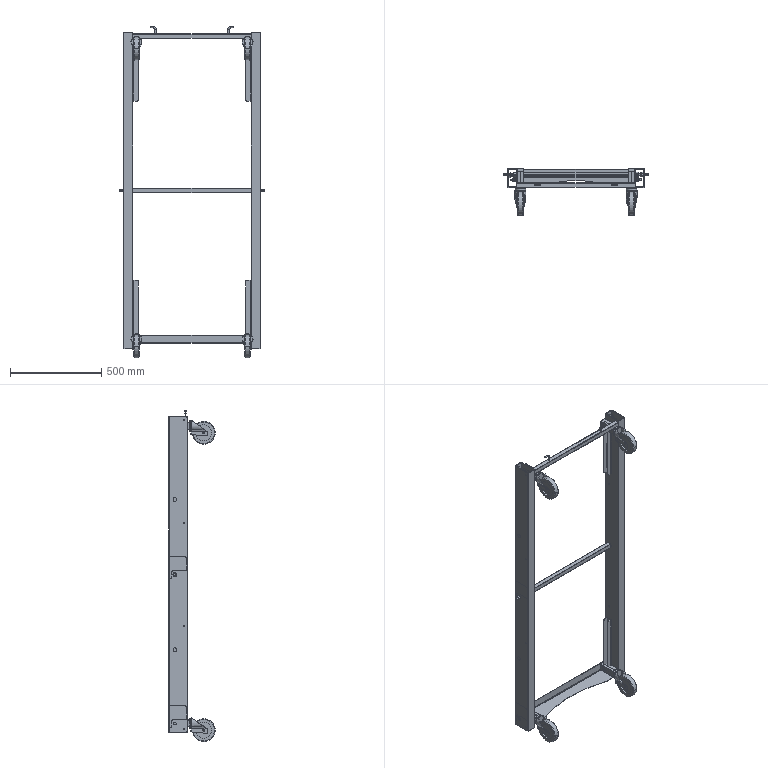Part | NX | features BREP 18 | 50 solids | 1032 faces | box 792.5 x 253.868 x 1813 mm | volume 6411804 mm3 | cylinder 519 | plane 435 | torus 44 | spline 24 | sphere 10 | commonest cylinder face diameters 3.175 x45 6.35 x36 3.81 x32 4.953 x32 8.89 x32 14.986 x32